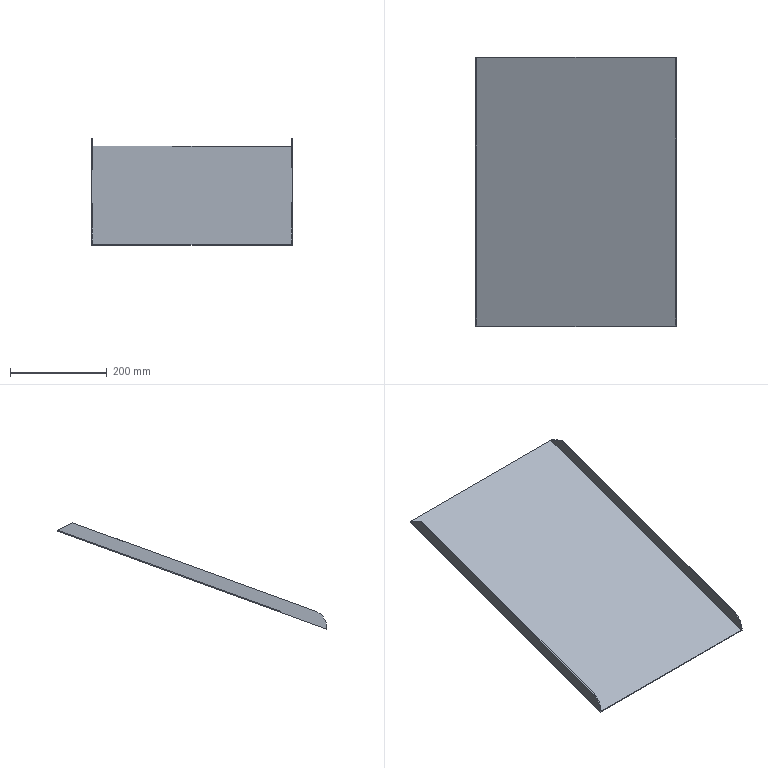Part | NX | features solid 2 | 1 solid | 14 faces | box 415 x 557.674 x 220.043 mm | volume 549316 mm3 | plane 11 | cylinder 2 | spline 1 | commonest cylinder face diameters 70 x2
STEP:
#1=CARTESIAN_POINT('',(-175.,-62.4,-217.894));
#2=VERTEX_POINT('',#1);
#3=CARTESIAN_POINT('',(-177.,-62.4,-217.894));
#4=VERTEX_POINT('',#3);
#5=CARTESIAN_POINT('',(-175.,-62.4,-217.894));
#6=DIRECTION('',(1.,0.,0.));
#7=VECTOR('',#6,1000.);
#8=LINE('',#5,#7);
#9=EDGE_CURVE('',#2,#4,#8,.F.);
#10=ORIENTED_EDGE('',*,*,#9,.F.);
#11=CARTESIAN_POINT('',(-590.,-62.338,-217.872));
#12=VERTEX_POINT('',#11);
#13=CARTESIAN_POINT('',(-590.,-62.338,-217.872));
#14=CARTESIAN_POINT('',(-451.667,-62.336,-217.871));
#15=CARTESIAN_POINT('',(-313.333,-62.288,-217.853));
#16=CARTESIAN_POINT('',(-175.,-62.4,-217.894));
#17=B_SPLINE_CURVE_WITH_KNOTS('',3,(#13,#14,#15,#16),.UNSPECIFIED.,.F.,.F.,(4,4),(0.,0.415),.UNSPECIFIED.);
#18=EDGE_CURVE('',#12,#2,#17,.T.);
#19=ORIENTED_EDGE('',*,*,#18,.F.);
#20=CARTESIAN_POINT('',(-588.,-62.338,-217.872));
#21=VERTEX_POINT('',#20);
#22=CARTESIAN_POINT('',(-590.,-62.338,-217.872));
#23=DIRECTION('',(1.,0.,0.));
#24=VECTOR('',#23,1000.);
#25=LINE('',#22,#24);
#26=EDGE_CURVE('',#12,#21,#25,.T.);
#27=ORIENTED_EDGE('',*,*,#26,.T.);
#28=CARTESIAN_POINT('',(-588.,-620.,-420.844));
#29=VERTEX_POINT('',#28);
#30=CARTESIAN_POINT('',(-588.,-62.338,-217.872));
#31=DIRECTION('',(0.,-0.9397,-0.342));
#32=VECTOR('',#31,1000.);
#33=LINE('',#30,#32);
#34=EDGE_CURVE('',#21,#29,#33,.T.);
#35=ORIENTED_EDGE('',*,*,#34,.T.);
#36=CARTESIAN_POINT('',(-177.,-620.,-420.844));
#37=VERTEX_POINT('',#36);
#38=CARTESIAN_POINT('',(-590.,-620.,-420.844));
#39=DIRECTION('',(1.,0.,0.));
#40=VECTOR('',#39,1000.);
#41=LINE('',#38,#40);
#42=EDGE_CURVE('',#29,#37,#41,.T.);
#43=ORIENTED_EDGE('',*,*,#42,.T.);
#44=CARTESIAN_POINT('',(-177.,-62.4,-217.894));
#45=DIRECTION('',(0.,-0.9397,-0.342));
#46=VECTOR('',#45,1000.);
#47=LINE('',#44,#46);
#48=EDGE_CURVE('',#4,#37,#47,.T.);
#49=ORIENTED_EDGE('',*,*,#48,.F.);
#50=EDGE_LOOP('',(#10,#19,#27,#35,#43,#49));
#51=FACE_BOUND('',#50,.T.);
#52=CARTESIAN_POINT('',(-590.,-63.022,-218.121));
#53=DIRECTION('',(0.,0.342,-0.9397));
#54=DIRECTION('',(-1.,0.,0.));
#55=AXIS2_PLACEMENT_3D('',#52,#53,#54);
#56=PLANE('',#55);
#57=ADVANCED_FACE('',(#51),#56,.F.);
#58=CARTESIAN_POINT('',(-588.,-620.,-418.747));
#59=VERTEX_POINT('',#58);
#60=CARTESIAN_POINT('',(-588.,-620.,-217.872));
#61=DIRECTION('',(0.,0.,-1.));
#62=VECTOR('',#61,1000.);
#63=LINE('',#60,#62);
#64=EDGE_CURVE('',#29,#59,#63,.F.);
#65=ORIENTED_EDGE('',*,*,#64,.T.);
#66=CARTESIAN_POINT('',(-590.,-620.,-418.747));
#67=VERTEX_POINT('',#66);
#68=CARTESIAN_POINT('',(-590.,-620.,-418.747));
#69=DIRECTION('',(-1.,0.,0.));
#70=VECTOR('',#69,1000.);
#71=LINE('',#68,#70);
#72=EDGE_CURVE('',#59,#67,#71,.T.);
#73=ORIENTED_EDGE('',*,*,#72,.T.);
#74=CARTESIAN_POINT('',(-590.,-620.,-422.972));
#75=VERTEX_POINT('',#74);
#76=CARTESIAN_POINT('',(-590.,-620.,-570.));
#77=DIRECTION('',(0.,0.,-1.));
#78=VECTOR('',#77,1000.);
#79=LINE('',#76,#78);
#80=EDGE_CURVE('',#67,#75,#79,.T.);
#81=ORIENTED_EDGE('',*,*,#80,.T.);
#82=CARTESIAN_POINT('',(-175.,-620.,-422.972));
#83=VERTEX_POINT('',#82);
#84=CARTESIAN_POINT('',(-590.,-620.,-422.972));
#85=DIRECTION('',(1.,0.,0.));
#86=VECTOR('',#85,1000.);
#87=LINE('',#84,#86);
#88=EDGE_CURVE('',#75,#83,#87,.T.);
#89=ORIENTED_EDGE('',*,*,#88,.T.);
#90=CARTESIAN_POINT('',(-175.,-620.,-418.747));
#91=VERTEX_POINT('',#90);
#92=CARTESIAN_POINT('',(-175.,-620.,-570.));
#93=DIRECTION('',(0.,0.,-1.));
#94=VECTOR('',#93,1000.);
#95=LINE('',#92,#94);
#96=EDGE_CURVE('',#91,#83,#95,.T.);
#97=ORIENTED_EDGE('',*,*,#96,.F.);
#98=CARTESIAN_POINT('',(-177.,-620.,-418.747));
#99=VERTEX_POINT('',#98);
#100=CARTESIAN_POINT('',(50.,-620.,-418.747));
#101=DIRECTION('',(-1.,0.,0.));
#102=VECTOR('',#101,1000.);
#103=LINE('',#100,#102);
#104=EDGE_CURVE('',#91,#99,#103,.T.);
#105=ORIENTED_EDGE('',*,*,#104,.T.);
#106=CARTESIAN_POINT('',(-177.,-620.,-570.));
#107=DIRECTION('',(0.,0.,1.));
#108=VECTOR('',#107,1000.);
#109=LINE('',#106,#108);
#110=EDGE_CURVE('',#37,#99,#109,.T.);
#111=ORIENTED_EDGE('',*,*,#110,.F.);
#112=ORIENTED_EDGE('',*,*,#42,.F.);
#113=EDGE_LOOP('',(#65,#73,#81,#89,#97,#105,#111,#112));
#114=FACE_BOUND('',#113,.T.);
#115=CARTESIAN_POINT('',(50.,-620.,-570.));
#116=DIRECTION('',(0.,1.,0.));
#117=DIRECTION('',(-1.,0.,0.));
#118=AXIS2_PLACEMENT_3D('',#115,#116,#117);
#119=PLANE('',#118);
#120=ADVANCED_FACE('',(#114),#119,.F.);
#121=CARTESIAN_POINT('',(-175.,-62.4,-220.023));
#122=VERTEX_POINT('',#121);
#123=CARTESIAN_POINT('',(-175.,-62.4,-219.06));
#124=DIRECTION('',(0.,0.,1.));
#125=VECTOR('',#124,1000.);
#126=LINE('',#123,#125);
#127=EDGE_CURVE('',#2,#122,#126,.F.);
#128=ORIENTED_EDGE('',*,*,#127,.F.);
#129=CARTESIAN_POINT('',(-175.,-94.443,-202.952));
#130=VERTEX_POINT('',#129);
#131=CARTESIAN_POINT('',(-175.,-62.824,-217.696));
#132=DIRECTION('',(0.,0.9063,-0.4226));
#133=VECTOR('',#132,1000.);
#134=LINE('',#131,#133);
#135=EDGE_CURVE('',#2,#130,#134,.F.);
#136=ORIENTED_EDGE('',*,*,#135,.T.);
#137=CARTESIAN_POINT('',(-175.,-596.971,-385.858));
#138=VERTEX_POINT('',#137);
#139=CARTESIAN_POINT('',(-175.,-70.95,-194.402));
#140=DIRECTION('',(0.,-0.9397,-0.342));
#141=VECTOR('',#140,1000.);
#142=LINE('',#139,#141);
#143=EDGE_CURVE('',#130,#138,#142,.T.);
#144=ORIENTED_EDGE('',*,*,#143,.T.);
#145=CARTESIAN_POINT('',(-175.,-585.,-418.747));
#146=DIRECTION('',(1.,0.,0.));
#147=DIRECTION('',(0.,0.,-1.));
#148=AXIS2_PLACEMENT_3D('',#145,#146,#147);
#149=CIRCLE('',#148,35.);
#150=EDGE_CURVE('',#138,#91,#149,.T.);
#151=ORIENTED_EDGE('',*,*,#150,.T.);
#152=ORIENTED_EDGE('',*,*,#96,.T.);
#153=CARTESIAN_POINT('',(-175.,-62.338,-220.));
#154=DIRECTION('',(0.,-0.9397,-0.342));
#155=VECTOR('',#154,1000.);
#156=LINE('',#153,#155);
#157=EDGE_CURVE('',#122,#83,#156,.T.);
#158=ORIENTED_EDGE('',*,*,#157,.F.);
#159=EDGE_LOOP('',(#128,#136,#144,#151,#152,#158));
#160=FACE_BOUND('',#159,.T.);
#161=CARTESIAN_POINT('',(-175.,-63.022,-218.121));
#162=DIRECTION('',(1.,0.,0.));
#163=DIRECTION('',(0.,0.,-1.));
#164=AXIS2_PLACEMENT_3D('',#161,#162,#163);
#165=PLANE('',#164);
#166=ADVANCED_FACE('',(#160),#165,.T.);
#167=CARTESIAN_POINT('',(-590.,-62.338,-220.));
#168=VERTEX_POINT('',#167);
#169=CARTESIAN_POINT('',(-590.,-62.338,-220.));
#170=CARTESIAN_POINT('',(-451.667,-62.336,-219.999));
#171=CARTESIAN_POINT('',(-313.333,-62.288,-219.982));
#172=CARTESIAN_POINT('',(-175.,-62.4,-220.023));
#173=B_SPLINE_CURVE_WITH_KNOTS('',3,(#169,#170,#171,#172),.UNSPECIFIED.,.F.,.F.,(4,4),(0.,0.415),.UNSPECIFIED.);
#174=EDGE_CURVE('',#168,#122,#173,.T.);
#175=ORIENTED_EDGE('',*,*,#174,.F.);
#176=CARTESIAN_POINT('',(-590.,-62.338,-219.06));
#177=DIRECTION('',(0.,0.,1.));
#178=VECTOR('',#177,1000.);
#179=LINE('',#176,#178);
#180=EDGE_CURVE('',#12,#168,#179,.F.);
#181=ORIENTED_EDGE('',*,*,#180,.F.);
#182=ORIENTED_EDGE('',*,*,#18,.T.);
#183=ORIENTED_EDGE('',*,*,#127,.T.);
#184=EDGE_LOOP('',(#175,#181,#182,#183));
#185=FACE_BOUND('',#184,.T.);
#186=CARTESIAN_POINT('',(-590.,-62.338,-220.036));
#187=CARTESIAN_POINT('',(-590.,-62.338,-217.852));
#188=CARTESIAN_POINT('',(-562.761,-62.338,-220.036));
#189=CARTESIAN_POINT('',(-562.761,-62.338,-217.852));
#190=CARTESIAN_POINT('',(-530.982,-62.337,-220.036));
#191=CARTESIAN_POINT('',(-530.982,-62.337,-217.852));
#192=CARTESIAN_POINT('',(-496.934,-62.337,-220.036));
#193=CARTESIAN_POINT('',(-496.934,-62.337,-217.852));
#194=CARTESIAN_POINT('',(-487.854,-62.337,-220.036));
#195=CARTESIAN_POINT('',(-487.854,-62.337,-217.852));
#196=CARTESIAN_POINT('',(-481.044,-62.337,-220.036));
#197=CARTESIAN_POINT('',(-481.044,-62.337,-217.852));
#198=CARTESIAN_POINT('',(-474.235,-62.337,-220.036));
#199=CARTESIAN_POINT('',(-474.235,-62.337,-217.852));
#200=CARTESIAN_POINT('',(-468.56,-62.337,-220.036));
#201=CARTESIAN_POINT('',(-468.56,-62.337,-217.852));
#202=CARTESIAN_POINT('',(-464.02,-62.337,-220.036));
#203=CARTESIAN_POINT('',(-464.02,-62.337,-217.852));
#204=CARTESIAN_POINT('',(-460.615,-62.337,-220.036));
#205=CARTESIAN_POINT('',(-460.615,-62.337,-217.852));
#206=CARTESIAN_POINT('',(-457.778,-62.337,-220.036));
#207=CARTESIAN_POINT('',(-457.778,-62.337,-217.852));
#208=CARTESIAN_POINT('',(-455.509,-62.337,-220.036));
#209=CARTESIAN_POINT('',(-455.509,-62.337,-217.852));
#210=CARTESIAN_POINT('',(-454.087,-62.337,-220.036));
#211=CARTESIAN_POINT('',(-454.087,-62.337,-217.852));
#212=CARTESIAN_POINT('',(-453.099,-62.337,-220.036));
#213=CARTESIAN_POINT('',(-453.099,-62.337,-217.852));
#214=CARTESIAN_POINT('',(-452.524,-62.337,-220.036));
#215=CARTESIAN_POINT('',(-452.524,-62.337,-217.852));
#216=CARTESIAN_POINT('',(-452.121,-62.337,-220.036));
#217=CARTESIAN_POINT('',(-452.121,-62.337,-217.852));
#218=CARTESIAN_POINT('',(-451.291,-62.337,-220.036));
#219=CARTESIAN_POINT('',(-451.291,-62.337,-217.852));
#220=CARTESIAN_POINT('',(-450.337,-62.337,-220.036));
#221=CARTESIAN_POINT('',(-450.337,-62.337,-217.852));
#222=CARTESIAN_POINT('',(-449.098,-62.337,-220.036));
#223=CARTESIAN_POINT('',(-449.098,-62.337,-217.852));
#224=CARTESIAN_POINT('',(-447.64,-62.337,-220.036));
#225=CARTESIAN_POINT('',(-447.64,-62.337,-217.852));
#226=CARTESIAN_POINT('',(-445.698,-62.337,-220.036));
#227=CARTESIAN_POINT('',(-445.698,-62.337,-217.852));
#228=CARTESIAN_POINT('',(-442.328,-62.337,-220.036));
#229=CARTESIAN_POINT('',(-442.328,-62.337,-217.852));
#230=CARTESIAN_POINT('',(-437.585,-62.337,-220.036));
#231=CARTESIAN_POINT('',(-437.585,-62.337,-217.852));
#232=CARTESIAN_POINT('',(-430.151,-62.337,-220.036));
#233=CARTESIAN_POINT('',(-430.151,-62.337,-217.852));
#234=CARTESIAN_POINT('',(-421.148,-62.337,-220.036));
#235=CARTESIAN_POINT('',(-421.148,-62.337,-217.852));
#236=CARTESIAN_POINT('',(-410.808,-62.337,-220.036));
#237=CARTESIAN_POINT('',(-410.808,-62.337,-217.852));
#238=CARTESIAN_POINT('',(-400.931,-62.336,-220.036));
#239=CARTESIAN_POINT('',(-400.931,-62.336,-217.852));
#240=CARTESIAN_POINT('',(-382.103,-62.336,-220.036));
#241=CARTESIAN_POINT('',(-382.103,-62.336,-217.852));
#242=CARTESIAN_POINT('',(-362.838,-62.336,-220.036));
#243=CARTESIAN_POINT('',(-362.838,-62.336,-217.852));
#244=CARTESIAN_POINT('',(-339.95,-62.334,-220.036));
#245=CARTESIAN_POINT('',(-339.95,-62.334,-217.852));
#246=CARTESIAN_POINT('',(-327.171,-62.333,-220.036));
#247=CARTESIAN_POINT('',(-327.171,-62.333,-217.852));
#248=CARTESIAN_POINT('',(-317.094,-62.332,-220.036));
#249=CARTESIAN_POINT('',(-317.094,-62.332,-217.852));
#250=CARTESIAN_POINT('',(-312.866,-62.331,-220.036));
#251=CARTESIAN_POINT('',(-312.866,-62.331,-217.852));
#252=CARTESIAN_POINT('',(-309.821,-62.331,-220.036));
#253=CARTESIAN_POINT('',(-309.821,-62.331,-217.852));
#254=CARTESIAN_POINT('',(-308.415,-62.33,-220.036));
#255=CARTESIAN_POINT('',(-308.415,-62.33,-217.852));
#256=CARTESIAN_POINT('',(-307.124,-62.33,-220.036));
#257=CARTESIAN_POINT('',(-307.124,-62.33,-217.852));
#258=CARTESIAN_POINT('',(-306.145,-62.33,-220.036));
#259=CARTESIAN_POINT('',(-306.145,-62.33,-217.852));
#260=CARTESIAN_POINT('',(-305.42,-62.33,-220.036));
#261=CARTESIAN_POINT('',(-305.42,-62.33,-217.852));
#262=CARTESIAN_POINT('',(-304.991,-62.329,-220.036));
#263=CARTESIAN_POINT('',(-304.991,-62.329,-217.852));
#264=CARTESIAN_POINT('',(-304.662,-62.329,-220.036));
#265=CARTESIAN_POINT('',(-304.662,-62.329,-217.852));
#266=CARTESIAN_POINT('',(-304.425,-62.329,-220.036));
#267=CARTESIAN_POINT('',(-304.425,-62.329,-217.852));
#268=CARTESIAN_POINT('',(-304.223,-62.329,-220.036));
#269=CARTESIAN_POINT('',(-304.223,-62.329,-217.852));
#270=CARTESIAN_POINT('',(-304.107,-62.329,-220.036));
#271=CARTESIAN_POINT('',(-304.107,-62.329,-217.852));
#272=CARTESIAN_POINT('',(-304.007,-62.329,-220.036));
#273=CARTESIAN_POINT('',(-304.007,-62.329,-217.852));
#274=CARTESIAN_POINT('',(-304.028,-62.329,-220.036));
#275=CARTESIAN_POINT('',(-304.028,-62.329,-217.852));
#276=CARTESIAN_POINT('',(-303.685,-62.329,-220.036));
#277=CARTESIAN_POINT('',(-303.685,-62.329,-217.852));
#278=CARTESIAN_POINT('',(-303.273,-62.329,-220.036));
#279=CARTESIAN_POINT('',(-303.273,-62.329,-217.852));
#280=CARTESIAN_POINT('',(-302.535,-62.328,-220.036));
#281=CARTESIAN_POINT('',(-302.535,-62.328,-217.852));
#282=CARTESIAN_POINT('',(-301.503,-62.328,-220.036));
#283=CARTESIAN_POINT('',(-301.503,-62.328,-217.852));
#284=CARTESIAN_POINT('',(-300.28,-62.328,-220.036));
#285=CARTESIAN_POINT('',(-300.28,-62.328,-217.852));
#286=CARTESIAN_POINT('',(-298.676,-62.327,-220.036));
#287=CARTESIAN_POINT('',(-298.676,-62.327,-217.852));
#288=CARTESIAN_POINT('',(-296.719,-62.326,-220.036));
#289=CARTESIAN_POINT('',(-296.719,-62.326,-217.852));
#290=CARTESIAN_POINT('',(-293.691,-62.325,-220.036));
#291=CARTESIAN_POINT('',(-293.691,-62.325,-217.852));
#292=CARTESIAN_POINT('',(-290.097,-62.324,-220.036));
#293=CARTESIAN_POINT('',(-290.097,-62.324,-217.852));
#294=CARTESIAN_POINT('',(-286.092,-62.323,-220.036));
#295=CARTESIAN_POINT('',(-286.092,-62.323,-217.852));
#296=CARTESIAN_POINT('',(-282.394,-62.322,-220.036));
#297=CARTESIAN_POINT('',(-282.394,-62.322,-217.852));
#298=CARTESIAN_POINT('',(-279.004,-62.322,-220.036));
#299=CARTESIAN_POINT('',(-279.004,-62.322,-217.852));
#300=CARTESIAN_POINT('',(-275.921,-62.322,-220.036));
#301=CARTESIAN_POINT('',(-275.921,-62.322,-217.852));
#302=CARTESIAN_POINT('',(-273.145,-62.322,-220.036));
#303=CARTESIAN_POINT('',(-273.145,-62.322,-217.852));
#304=CARTESIAN_POINT('',(-271.086,-62.323,-220.036));
#305=CARTESIAN_POINT('',(-271.086,-62.323,-217.852));
#306=CARTESIAN_POINT('',(-269.596,-62.323,-220.036));
#307=CARTESIAN_POINT('',(-269.596,-62.323,-217.852));
#308=CARTESIAN_POINT('',(-268.543,-62.324,-220.036));
#309=CARTESIAN_POINT('',(-268.543,-62.324,-217.852));
#310=CARTESIAN_POINT('',(-267.768,-62.324,-220.036));
#311=CARTESIAN_POINT('',(-267.768,-62.324,-217.852));
#312=CARTESIAN_POINT('',(-267.183,-62.325,-220.036));
#313=CARTESIAN_POINT('',(-267.183,-62.325,-217.852));
#314=CARTESIAN_POINT('',(-267.003,-62.325,-220.036));
#315=CARTESIAN_POINT('',(-267.003,-62.325,-217.852));
#316=CARTESIAN_POINT('',(-266.734,-62.325,-220.036));
#317=CARTESIAN_POINT('',(-266.734,-62.325,-217.852));
#318=CARTESIAN_POINT('',(-266.367,-62.326,-220.036));
#319=CARTESIAN_POINT('',(-266.367,-62.326,-217.852));
#320=CARTESIAN_POINT('',(-265.944,-62.326,-220.036));
#321=CARTESIAN_POINT('',(-265.944,-62.326,-217.852));
#322=CARTESIAN_POINT('',(-265.252,-62.327,-220.036));
#323=CARTESIAN_POINT('',(-265.252,-62.327,-217.852));
#324=CARTESIAN_POINT('',(-264.065,-62.327,-220.036));
#325=CARTESIAN_POINT('',(-264.065,-62.327,-217.852));
#326=CARTESIAN_POINT('',(-262.401,-62.329,-220.036));
#327=CARTESIAN_POINT('',(-262.401,-62.329,-217.852));
#328=CARTESIAN_POINT('',(-260.466,-62.33,-220.036));
#329=CARTESIAN_POINT('',(-260.466,-62.33,-217.852));
#330=CARTESIAN_POINT('',(-257.963,-62.333,-220.036));
#331=CARTESIAN_POINT('',(-257.963,-62.333,-217.852));
#332=CARTESIAN_POINT('',(-254.984,-62.335,-220.036));
#333=CARTESIAN_POINT('',(-254.984,-62.335,-217.852));
#334=CARTESIAN_POINT('',(-251.645,-62.338,-220.036));
#335=CARTESIAN_POINT('',(-251.645,-62.338,-217.852));
#336=CARTESIAN_POINT('',(-248.546,-62.34,-220.036));
#337=CARTESIAN_POINT('',(-248.546,-62.34,-217.852));
#338=CARTESIAN_POINT('',(-245.676,-62.343,-220.036));
#339=CARTESIAN_POINT('',(-245.676,-62.343,-217.852));
#340=CARTESIAN_POINT('',(-242.201,-62.345,-220.036));
#341=CARTESIAN_POINT('',(-242.201,-62.345,-217.852));
#342=CARTESIAN_POINT('',(-237.83,-62.349,-220.036));
#343=CARTESIAN_POINT('',(-237.83,-62.349,-217.852));
#344=CARTESIAN_POINT('',(-232.596,-62.353,-220.036));
#345=CARTESIAN_POINT('',(-232.596,-62.353,-217.852));
#346=CARTESIAN_POINT('',(-225.614,-62.359,-220.036));
#347=CARTESIAN_POINT('',(-225.614,-62.359,-217.852));
#348=CARTESIAN_POINT('',(-216.888,-62.366,-220.036));
#349=CARTESIAN_POINT('',(-216.888,-62.366,-217.852));
#350=CARTESIAN_POINT('',(-206.416,-62.374,-220.036));
#351=CARTESIAN_POINT('',(-206.416,-62.374,-217.852));
#352=CARTESIAN_POINT('',(-192.453,-62.386,-220.036));
#353=CARTESIAN_POINT('',(-192.453,-62.386,-217.852));
#354=CARTESIAN_POINT('',(-181.981,-62.394,-220.036));
#355=CARTESIAN_POINT('',(-181.981,-62.394,-217.852));
#356=CARTESIAN_POINT('',(-175.,-62.4,-220.036));
#357=CARTESIAN_POINT('',(-175.,-62.4,-217.852));
#358=B_SPLINE_SURFACE_WITH_KNOTS('',3,1,((#186,#187),(#188,#189),(#190,#191),(#192,#193),(#194,#195),(#196,#197),(#198,#199),(#200,#201),(#202,#203),(#204,#205),(#206,#207),(#208,#209),(#210,#211),(#212,#213),(#214,#215),(#216,#217),(#218,#219),(#220,#221),(#222,#223),(#224,#225),(#226,#227),(#228,#229),(#230,#231),(#232,#233),(#234,#235),(#236,#237),(#238,#239),(#240,#241),(#242,#243),(#244,#245),(#246,#247),(#248,#249),(#250,#251),(#252,#253),(#254,#255),(#256,#257),(#258,#259),(#260,#261),(#262,#263),(#264,#265),(#266,#267),(#268,#269),(#270,#271),(#272,#273),(#274,#275),(#276,#277),(#278,#279),(#280,#281),(#282,#283),(#284,#285),(#286,#287),(#288,#289),(#290,#291),(#292,#293),(#294,#295),(#296,#297),(#298,#299),(#300,#301),(#302,#303),(#304,#305),(#306,#307),(#308,#309),(#310,#311),(#312,#313),(#314,#315),(#316,#317),(#318,#319),(#320,#321),(#322,#323),(#324,#325),(#326,#327),(#328,#329),(#330,#331),(#332,#333),(#334,#335),(#336,#337),(#338,#339),(#340,#341),(#342,#343),(#344,#345),(#346,#347),(#348,#349),(#350,#351),(#352,#353),(#354,#355),(#356,#357)),.UNSPECIFIED.,.F.,.F.,.F.,(4,1,1,1,1,1,1,1,1,1,1,1,1,1,1,1,1,1,1,1,1,1,1,1,1,1,1,1,1,1,1,1,1,1,1,1,1,1,1,1,1,1,1,1,1,1,1,1,1,1,1,1,1,1,1,1,1,1,1,1,1,1,1,1,1,1,1,1,1,1,1,1,1,1,1,1,1,1,1,1,1,1,1,4),(2,2),(-0.3915,-0.0626,-0.007784,0.01962,0.04703,0.07444,0.1018,0.1156,0.1293,0.143,0.1498,0.1567,0.1601,0.1618,0.1635,0.1652,0.1669,0.1704,0.1738,0.1772,0.1841,0.1978,0.2115,0.2389,0.2663,0.2937,0.3211,0.4308,0.4856,0.5952,0.6226,0.6774,0.6911,0.7048,0.7185,0.7322,0.7391,0.746,0.7494,0.7528,0.7562,0.7579,0.7588,0.7597,0.7605,0.7614,0.7631,0.7665,0.7699,0.7734,0.7802,0.7871,0.8008,0.8145,0.8282,0.8419,0.8556,0.8693,0.883,0.8898,0.8967,0.9035,0.907,0.9087,0.9095,0.9104,0.9121,0.9138,0.9173,0.9241,0.931,0.9378,0.9515,0.9652,0.9789,0.9926,1.006,1.034,1.061,1.089,1.143,1.198,1.253,1.363),(0.,1.),.UNSPECIFIED.);
#359=ADVANCED_FACE('',(#185),#358,.F.);
#360=CARTESIAN_POINT('',(-590.,-94.381,-202.93));
#361=VERTEX_POINT('',#360);
#362=CARTESIAN_POINT('',(-590.,-596.971,-385.858));
#363=VERTEX_POINT('',#362);
#364=CARTESIAN_POINT('',(-590.,-70.888,-194.379));
#365=DIRECTION('',(0.,-0.9397,-0.342));
#366=VECTOR('',#365,1000.);
#367=LINE('',#364,#366);
#368=EDGE_CURVE('',#361,#363,#367,.T.);
#369=ORIENTED_EDGE('',*,*,#368,.F.);
#370=CARTESIAN_POINT('',(-590.,-62.338,-217.872));
#371=DIRECTION('',(0.,-0.9063,0.4226));
#372=VECTOR('',#371,1000.);
#373=LINE('',#370,#372);
#374=EDGE_CURVE('',#361,#12,#373,.F.);
#375=ORIENTED_EDGE('',*,*,#374,.T.);
#376=ORIENTED_EDGE('',*,*,#180,.T.);
#377=CARTESIAN_POINT('',(-590.,-62.338,-220.));
#378=DIRECTION('',(0.,-0.9397,-0.342));
#379=VECTOR('',#378,1000.);
#380=LINE('',#377,#379);
#381=EDGE_CURVE('',#168,#75,#380,.T.);
#382=ORIENTED_EDGE('',*,*,#381,.T.);
#383=ORIENTED_EDGE('',*,*,#80,.F.);
#384=CARTESIAN_POINT('',(-590.,-585.,-418.747));
#385=DIRECTION('',(1.,0.,0.));
#386=DIRECTION('',(0.,0.,-1.));
#387=AXIS2_PLACEMENT_3D('',#384,#385,#386);
#388=CIRCLE('',#387,35.);
#389=EDGE_CURVE('',#67,#363,#388,.F.);
#390=ORIENTED_EDGE('',*,*,#389,.T.);
#391=EDGE_LOOP('',(#369,#375,#376,#382,#383,#390));
#392=FACE_BOUND('',#391,.T.);
#393=CARTESIAN_POINT('',(-590.,-63.022,-218.121));
#394=DIRECTION('',(1.,0.,0.));
#395=DIRECTION('',(0.,0.,-1.));
#396=AXIS2_PLACEMENT_3D('',#393,#394,#395);
#397=PLANE('',#396);
#398=ADVANCED_FACE('',(#392),#397,.F.);
#399=ORIENTED_EDGE('',*,*,#88,.F.);
#400=ORIENTED_EDGE('',*,*,#381,.F.);
#401=ORIENTED_EDGE('',*,*,#174,.T.);
#402=ORIENTED_EDGE('',*,*,#157,.T.);
#403=EDGE_LOOP('',(#399,#400,#401,#402));
#404=FACE_BOUND('',#403,.T.);
#405=CARTESIAN_POINT('',(-590.,-62.338,-220.));
#406=DIRECTION('',(0.,0.342,-0.9397));
#407=DIRECTION('',(-1.,0.,0.));
#408=AXIS2_PLACEMENT_3D('',#405,#406,#407);
#409=PLANE('',#408);
#410=ADVANCED_FACE('',(#404),#409,.T.);
#411=CARTESIAN_POINT('',(-588.,-94.381,-202.93));
#412=VERTEX_POINT('',#411);
#413=CARTESIAN_POINT('',(-588.,-596.971,-385.858));
#414=VERTEX_POINT('',#413);
#415=CARTESIAN_POINT('',(-588.,-70.888,-194.379));
#416=DIRECTION('',(0.,-0.9397,-0.342));
#417=VECTOR('',#416,1000.);
#418=LINE('',#415,#417);
#419=EDGE_CURVE('',#412,#414,#418,.T.);
#420=ORIENTED_EDGE('',*,*,#419,.F.);
#421=CARTESIAN_POINT('',(-590.,-94.381,-202.93));
#422=DIRECTION('',(1.,0.,0.));
#423=VECTOR('',#422,1000.);
#424=LINE('',#421,#423);
#425=EDGE_CURVE('',#412,#361,#424,.F.);
#426=ORIENTED_EDGE('',*,*,#425,.T.);
#427=ORIENTED_EDGE('',*,*,#368,.T.);
#428=CARTESIAN_POINT('',(-588.,-596.971,-385.858));
#429=DIRECTION('',(1.,0.,0.));
#430=VECTOR('',#429,1000.);
#431=LINE('',#428,#430);
#432=EDGE_CURVE('',#363,#414,#431,.T.);
#433=ORIENTED_EDGE('',*,*,#432,.T.);
#434=EDGE_LOOP('',(#420,#426,#427,#433));
#435=FACE_BOUND('',#434,.T.);
#436=CARTESIAN_POINT('',(-590.,-70.888,-194.379));
#437=DIRECTION('',(0.,0.342,-0.9397));
#438=DIRECTION('',(0.,-0.9397,-0.342));
#439=AXIS2_PLACEMENT_3D('',#436,#437,#438);
#440=PLANE('',#439);
#441=ADVANCED_FACE('',(#435),#440,.F.);
#442=ORIENTED_EDGE('',*,*,#34,.F.);
#443=CARTESIAN_POINT('',(-588.,-62.338,-217.872));
#444=DIRECTION('',(0.,0.9063,-0.4226));
#445=VECTOR('',#444,1000.);
#446=LINE('',#443,#445);
#447=EDGE_CURVE('',#21,#412,#446,.F.);
#448=ORIENTED_EDGE('',*,*,#447,.T.);
#449=ORIENTED_EDGE('',*,*,#419,.T.);
#450=CARTESIAN_POINT('',(-588.,-585.,-418.747));
#451=DIRECTION('',(-1.,0.,0.));
#452=DIRECTION('',(0.,0.,1.));
#453=AXIS2_PLACEMENT_3D('',#450,#451,#452);
#454=CIRCLE('',#453,35.);
#455=EDGE_CURVE('',#414,#59,#454,.F.);
#456=ORIENTED_EDGE('',*,*,#455,.T.);
#457=ORIENTED_EDGE('',*,*,#64,.F.);
#458=EDGE_LOOP('',(#442,#448,#449,#456,#457));
#459=FACE_BOUND('',#458,.T.);
#460=CARTESIAN_POINT('',(-588.,-62.338,-217.872));
#461=DIRECTION('',(-1.,0.,0.));
#462=DIRECTION('',(0.,0.,1.));
#463=AXIS2_PLACEMENT_3D('',#460,#461,#462);
#464=PLANE('',#463);
#465=ADVANCED_FACE('',(#459),#464,.F.);
#466=ORIENTED_EDGE('',*,*,#143,.F.);
#467=CARTESIAN_POINT('',(-177.,-94.443,-202.952));
#468=VERTEX_POINT('',#467);
#469=CARTESIAN_POINT('',(-175.,-94.443,-202.952));
#470=DIRECTION('',(-1.,0.,0.));
#471=VECTOR('',#470,1000.);
#472=LINE('',#469,#471);
#473=EDGE_CURVE('',#130,#468,#472,.T.);
#474=ORIENTED_EDGE('',*,*,#473,.T.);
#475=CARTESIAN_POINT('',(-177.,-596.971,-385.858));
#476=VERTEX_POINT('',#475);
#477=CARTESIAN_POINT('',(-177.,-70.95,-194.402));
#478=DIRECTION('',(0.,-0.9397,-0.342));
#479=VECTOR('',#478,1000.);
#480=LINE('',#477,#479);
#481=EDGE_CURVE('',#468,#476,#480,.T.);
#482=ORIENTED_EDGE('',*,*,#481,.T.);
#483=CARTESIAN_POINT('',(-175.,-596.971,-385.858));
#484=DIRECTION('',(-1.,0.,0.));
#485=VECTOR('',#484,1000.);
#486=LINE('',#483,#485);
#487=EDGE_CURVE('',#476,#138,#486,.F.);
#488=ORIENTED_EDGE('',*,*,#487,.T.);
#489=EDGE_LOOP('',(#466,#474,#482,#488));
#490=FACE_BOUND('',#489,.T.);
#491=CARTESIAN_POINT('',(-175.,-70.95,-194.402));
#492=DIRECTION('',(0.,0.342,-0.9397));
#493=DIRECTION('',(0.,-0.9397,-0.342));
#494=AXIS2_PLACEMENT_3D('',#491,#492,#493);
#495=PLANE('',#494);
#496=ADVANCED_FACE('',(#490),#495,.F.);
#497=ORIENTED_EDGE('',*,*,#481,.F.);
#498=CARTESIAN_POINT('',(-177.,-62.4,-217.894));
#499=DIRECTION('',(0.,-0.9063,0.4226));
#500=VECTOR('',#499,1000.);
#501=LINE('',#498,#500);
#502=EDGE_CURVE('',#468,#4,#501,.F.);
#503=ORIENTED_EDGE('',*,*,#502,.T.);
#504=ORIENTED_EDGE('',*,*,#48,.T.);
#505=ORIENTED_EDGE('',*,*,#110,.T.);
#506=CARTESIAN_POINT('',(-177.,-585.,-418.747));
#507=DIRECTION('',(-1.,0.,0.));
#508=DIRECTION('',(0.,0.,1.));
#509=AXIS2_PLACEMENT_3D('',#506,#507,#508);
#510=CIRCLE('',#509,35.);
#511=EDGE_CURVE('',#99,#476,#510,.T.);
#512=ORIENTED_EDGE('',*,*,#511,.T.);
#513=EDGE_LOOP('',(#497,#503,#504,#505,#512));
#514=FACE_BOUND('',#513,.T.);
#515=CARTESIAN_POINT('',(-177.,-62.4,-217.894));
#516=DIRECTION('',(-1.,0.,0.));
#517=DIRECTION('',(0.,0.,1.));
#518=AXIS2_PLACEMENT_3D('',#515,#516,#517);
#519=PLANE('',#518);
#520=ADVANCED_FACE('',(#514),#519,.T.);
#521=ORIENTED_EDGE('',*,*,#150,.F.);
#522=ORIENTED_EDGE('',*,*,#487,.F.);
#523=ORIENTED_EDGE('',*,*,#511,.F.);
#524=ORIENTED_EDGE('',*,*,#104,.F.);
#525=EDGE_LOOP('',(#521,#522,#523,#524));
#526=FACE_BOUND('',#525,.T.);
#527=CARTESIAN_POINT('',(50.,-585.,-418.747));
#528=DIRECTION('',(-1.,0.,0.));
#529=DIRECTION('',(0.,0.,1.));
#530=AXIS2_PLACEMENT_3D('',#527,#528,#529);
#531=CYLINDRICAL_SURFACE('',#530,35.);
#532=ADVANCED_FACE('',(#526),#531,.T.);
#533=ORIENTED_EDGE('',*,*,#389,.F.);
#534=ORIENTED_EDGE('',*,*,#72,.F.);
#535=ORIENTED_EDGE('',*,*,#455,.F.);
#536=ORIENTED_EDGE('',*,*,#432,.F.);
#537=EDGE_LOOP('',(#533,#534,#535,#536));
#538=FACE_BOUND('',#537,.T.);
#539=CARTESIAN_POINT('',(-590.,-585.,-418.747));
#540=DIRECTION('',(1.,0.,0.));
#541=DIRECTION('',(0.,0.,-1.));
#542=AXIS2_PLACEMENT_3D('',#539,#540,#541);
#543=CYLINDRICAL_SURFACE('',#542,35.);
#544=ADVANCED_FACE('',(#538),#543,.T.);
#545=ORIENTED_EDGE('',*,*,#135,.F.);
#546=ORIENTED_EDGE('',*,*,#9,.T.);
#547=ORIENTED_EDGE('',*,*,#502,.F.);
#548=ORIENTED_EDGE('',*,*,#473,.F.);
#549=EDGE_LOOP('',(#545,#546,#547,#548));
#550=FACE_BOUND('',#549,.T.);
#551=CARTESIAN_POINT('',(-175.,-94.443,-202.952));
#552=DIRECTION('',(0.,-0.4226,-0.9063));
#553=DIRECTION('',(0.,0.9063,-0.4226));
#554=AXIS2_PLACEMENT_3D('',#551,#552,#553);
#555=PLANE('',#554);
#556=ADVANCED_FACE('',(#550),#555,.F.);
#557=ORIENTED_EDGE('',*,*,#374,.F.);
#558=ORIENTED_EDGE('',*,*,#425,.F.);
#559=ORIENTED_EDGE('',*,*,#447,.F.);
#560=ORIENTED_EDGE('',*,*,#26,.F.);
#561=EDGE_LOOP('',(#557,#558,#559,#560));
#562=FACE_BOUND('',#561,.T.);
#563=CARTESIAN_POINT('',(-590.,-62.338,-217.872));
#564=DIRECTION('',(0.,-0.4226,-0.9063));
#565=DIRECTION('',(0.,0.9063,-0.4226));
#566=AXIS2_PLACEMENT_3D('',#563,#564,#565);
#567=PLANE('',#566);
#568=ADVANCED_FACE('',(#562),#567,.F.);
#569=CLOSED_SHELL('',(#57,#120,#166,#359,#398,#410,#441,#465,#496,#520,#532,#544,#556,#568));
#570=MANIFOLD_SOLID_BREP('',#569);
#571=(LENGTH_UNIT()NAMED_UNIT(*)SI_UNIT(.MILLI.,.METRE.));
#572=UNCERTAINTY_MEASURE_WITH_UNIT(LENGTH_MEASURE(0.0508),#571,'','');
#573=(NAMED_UNIT(*)PLANE_ANGLE_UNIT()SI_UNIT($,.RADIAN.));
#574=(NAMED_UNIT(*)SI_UNIT($,.STERADIAN.)SOLID_ANGLE_UNIT());
#575=(GEOMETRIC_REPRESENTATION_CONTEXT(3)GLOBAL_UNCERTAINTY_ASSIGNED_CONTEXT((#572))GLOBAL_UNIT_ASSIGNED_CONTEXT((#571,#573,#574))REPRESENTATION_CONTEXT('',''));
#576=ADVANCED_BREP_SHAPE_REPRESENTATION('',(#570),#575);